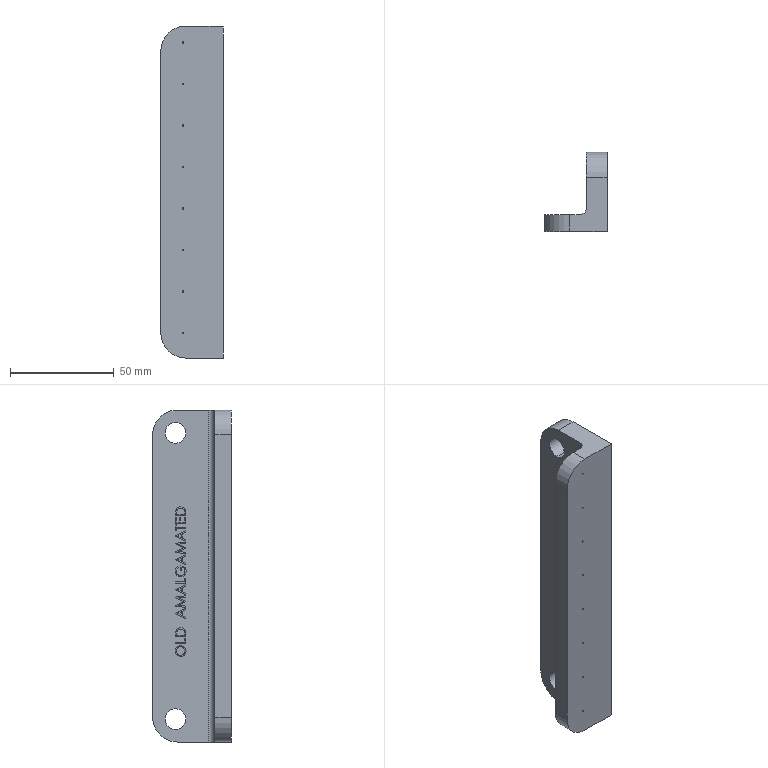Part | SolidWorks | features ICE 3, Fillet 2, Extrusion 1 | 1 solid | 203 faces | box 30 x 38 x 160 mm | volume 83802 mm3 | plane 147 | spline 31 | cylinder 25 | commonest cylinder face diameters 0.58 x16 10 x4 24 x4 6 x1